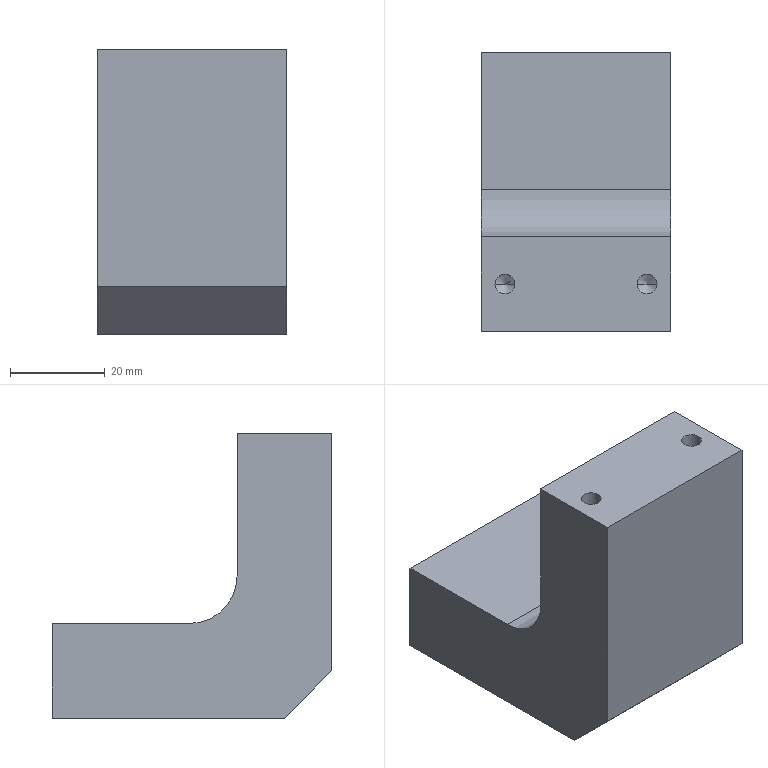Part | SolidWorks | features 3DProfileFeature 2, HoleWzd 2, Chamfer 1, Extrusion 1, Fillet 1, ICE 1 | 1 solid | 26 faces | box 40 x 59 x 60 mm | volume 77348 mm3 | cylinder 9 | plane 9 | cone 8 | commonest cylinder face diameters 4.2 x8 20 x1
STEP:
#1=CARTESIAN_POINT('',(-17.1,10.,17.6));
#2=VERTEX_POINT('',#1);
#3=CARTESIAN_POINT('',(-12.9,10.,17.6));
#4=VERTEX_POINT('',#3);
#5=CARTESIAN_POINT('',(-15.,10.,17.6));
#6=DIRECTION('',(0.,0.,1.));
#7=DIRECTION('',(1.,0.,0.));
#8=AXIS2_PLACEMENT_3D('',#5,#6,#7);
#9=CIRCLE('',#8,2.1);
#10=EDGE_CURVE('',#2,#4,#9,.T.);
#11=ORIENTED_EDGE('',*,*,#10,.F.);
#12=CARTESIAN_POINT('',(-17.1,10.,30.));
#13=VERTEX_POINT('',#12);
#14=CARTESIAN_POINT('',(-17.1,10.,30.));
#15=DIRECTION('',(0.,0.,1.));
#16=VECTOR('',#15,1000.);
#17=LINE('',#14,#16);
#18=EDGE_CURVE('',#2,#13,#17,.T.);
#19=ORIENTED_EDGE('',*,*,#18,.T.);
#20=CARTESIAN_POINT('',(-12.9,10.,30.));
#21=VERTEX_POINT('',#20);
#22=CARTESIAN_POINT('',(-15.,10.,30.));
#23=DIRECTION('',(0.,0.,1.));
#24=DIRECTION('',(1.,0.,0.));
#25=AXIS2_PLACEMENT_3D('',#22,#23,#24);
#26=CIRCLE('',#25,2.1);
#27=EDGE_CURVE('',#13,#21,#26,.T.);
#28=ORIENTED_EDGE('',*,*,#27,.T.);
#29=CARTESIAN_POINT('',(-12.9,10.,30.));
#30=DIRECTION('',(0.,0.,1.));
#31=VECTOR('',#30,1000.);
#32=LINE('',#29,#31);
#33=EDGE_CURVE('',#4,#21,#32,.T.);
#34=ORIENTED_EDGE('',*,*,#33,.F.);
#35=EDGE_LOOP('',(#11,#19,#28,#34));
#36=FACE_OUTER_BOUND('',#35,.T.);
#37=CARTESIAN_POINT('',(-15.,10.,30.));
#38=DIRECTION('',(0.,0.,1.));
#39=DIRECTION('',(1.,0.,0.));
#40=AXIS2_PLACEMENT_3D('',#37,#38,#39);
#41=CYLINDRICAL_SURFACE('',#40,2.1);
#42=ADVANCED_FACE('',(#36),#41,.F.);
#43=CARTESIAN_POINT('',(-15.,10.,16.338));
#44=VERTEX_POINT('',#43);
#45=CARTESIAN_POINT('',(-12.9,10.,17.6));
#46=DIRECTION('',(0.8572,0.,0.515));
#47=VECTOR('',#46,1000.);
#48=LINE('',#45,#47);
#49=EDGE_CURVE('',#44,#4,#48,.T.);
#50=ORIENTED_EDGE('',*,*,#49,.F.);
#51=CARTESIAN_POINT('',(-17.1,10.,17.6));
#52=DIRECTION('',(-0.8572,0.,0.515));
#53=VECTOR('',#52,1000.);
#54=LINE('',#51,#53);
#55=EDGE_CURVE('',#44,#2,#54,.T.);
#56=ORIENTED_EDGE('',*,*,#55,.T.);
#57=ORIENTED_EDGE('',*,*,#10,.T.);
#58=EDGE_LOOP('',(#50,#56,#57));
#59=FACE_OUTER_BOUND('',#58,.T.);
#60=CARTESIAN_POINT('',(-15.,10.,17.6));
#61=DIRECTION('',(0.,0.,1.));
#62=DIRECTION('',(1.,0.,0.));
#63=AXIS2_PLACEMENT_3D('',#60,#61,#62);
#64=CONICAL_SURFACE('',#63,2.1,1.03);
#65=ADVANCED_FACE('',(#59),#64,.F.);
#66=CARTESIAN_POINT('',(12.9,10.,17.6));
#67=VERTEX_POINT('',#66);
#68=CARTESIAN_POINT('',(17.1,10.,17.6));
#69=VERTEX_POINT('',#68);
#70=CARTESIAN_POINT('',(15.,10.,17.6));
#71=DIRECTION('',(0.,0.,1.));
#72=DIRECTION('',(1.,0.,0.));
#73=AXIS2_PLACEMENT_3D('',#70,#71,#72);
#74=CIRCLE('',#73,2.1);
#75=EDGE_CURVE('',#67,#69,#74,.T.);
#76=ORIENTED_EDGE('',*,*,#75,.F.);
#77=CARTESIAN_POINT('',(12.9,10.,30.));
#78=VERTEX_POINT('',#77);
#79=CARTESIAN_POINT('',(12.9,10.,30.));
#80=DIRECTION('',(0.,0.,1.));
#81=VECTOR('',#80,1000.);
#82=LINE('',#79,#81);
#83=EDGE_CURVE('',#67,#78,#82,.T.);
#84=ORIENTED_EDGE('',*,*,#83,.T.);
#85=CARTESIAN_POINT('',(17.1,10.,30.));
#86=VERTEX_POINT('',#85);
#87=CARTESIAN_POINT('',(15.,10.,30.));
#88=DIRECTION('',(0.,0.,1.));
#89=DIRECTION('',(1.,0.,0.));
#90=AXIS2_PLACEMENT_3D('',#87,#88,#89);
#91=CIRCLE('',#90,2.1);
#92=EDGE_CURVE('',#78,#86,#91,.T.);
#93=ORIENTED_EDGE('',*,*,#92,.T.);
#94=CARTESIAN_POINT('',(17.1,10.,30.));
#95=DIRECTION('',(0.,0.,1.));
#96=VECTOR('',#95,1000.);
#97=LINE('',#94,#96);
#98=EDGE_CURVE('',#69,#86,#97,.T.);
#99=ORIENTED_EDGE('',*,*,#98,.F.);
#100=EDGE_LOOP('',(#76,#84,#93,#99));
#101=FACE_OUTER_BOUND('',#100,.T.);
#102=CARTESIAN_POINT('',(15.,10.,30.));
#103=DIRECTION('',(0.,0.,1.));
#104=DIRECTION('',(1.,0.,0.));
#105=AXIS2_PLACEMENT_3D('',#102,#103,#104);
#106=CYLINDRICAL_SURFACE('',#105,2.1);
#107=ADVANCED_FACE('',(#101),#106,.F.);
#108=CARTESIAN_POINT('',(15.,10.,16.338));
#109=VERTEX_POINT('',#108);
#110=CARTESIAN_POINT('',(17.1,10.,17.6));
#111=DIRECTION('',(0.8572,0.,0.515));
#112=VECTOR('',#111,1000.);
#113=LINE('',#110,#112);
#114=EDGE_CURVE('',#109,#69,#113,.T.);
#115=ORIENTED_EDGE('',*,*,#114,.F.);
#116=CARTESIAN_POINT('',(12.9,10.,17.6));
#117=DIRECTION('',(-0.8572,0.,0.515));
#118=VECTOR('',#117,1000.);
#119=LINE('',#116,#118);
#120=EDGE_CURVE('',#109,#67,#119,.T.);
#121=ORIENTED_EDGE('',*,*,#120,.T.);
#122=ORIENTED_EDGE('',*,*,#75,.T.);
#123=EDGE_LOOP('',(#115,#121,#122));
#124=FACE_OUTER_BOUND('',#123,.T.);
#125=CARTESIAN_POINT('',(15.,10.,17.6));
#126=DIRECTION('',(0.,0.,1.));
#127=DIRECTION('',(1.,0.,0.));
#128=AXIS2_PLACEMENT_3D('',#125,#126,#127);
#129=CONICAL_SURFACE('',#128,2.1,1.03);
#130=ADVANCED_FACE('',(#124),#129,.F.);
#131=CARTESIAN_POINT('',(-14.,46.6,-22.1));
#132=VERTEX_POINT('',#131);
#133=CARTESIAN_POINT('',(-14.,46.6,-17.9));
#134=VERTEX_POINT('',#133);
#135=CARTESIAN_POINT('',(-14.,46.6,-20.));
#136=DIRECTION('',(0.,1.,0.));
#137=DIRECTION('',(0.,0.,1.));
#138=AXIS2_PLACEMENT_3D('',#135,#136,#137);
#139=CIRCLE('',#138,2.1);
#140=EDGE_CURVE('',#132,#134,#139,.T.);
#141=ORIENTED_EDGE('',*,*,#140,.F.);
#142=CARTESIAN_POINT('',(-14.,59.,-22.1));
#143=VERTEX_POINT('',#142);
#144=CARTESIAN_POINT('',(-14.,59.,-22.1));
#145=DIRECTION('',(0.,1.,0.));
#146=VECTOR('',#145,1000.);
#147=LINE('',#144,#146);
#148=EDGE_CURVE('',#132,#143,#147,.T.);
#149=ORIENTED_EDGE('',*,*,#148,.T.);
#150=CARTESIAN_POINT('',(-14.,59.,-17.9));
#151=VERTEX_POINT('',#150);
#152=CARTESIAN_POINT('',(-14.,59.,-20.));
#153=DIRECTION('',(0.,1.,0.));
#154=DIRECTION('',(0.,0.,1.));
#155=AXIS2_PLACEMENT_3D('',#152,#153,#154);
#156=CIRCLE('',#155,2.1);
#157=EDGE_CURVE('',#143,#151,#156,.T.);
#158=ORIENTED_EDGE('',*,*,#157,.T.);
#159=CARTESIAN_POINT('',(-14.,59.,-17.9));
#160=DIRECTION('',(0.,1.,0.));
#161=VECTOR('',#160,1000.);
#162=LINE('',#159,#161);
#163=EDGE_CURVE('',#134,#151,#162,.T.);
#164=ORIENTED_EDGE('',*,*,#163,.F.);
#165=EDGE_LOOP('',(#141,#149,#158,#164));
#166=FACE_OUTER_BOUND('',#165,.T.);
#167=CARTESIAN_POINT('',(-14.,59.,-20.));
#168=DIRECTION('',(0.,1.,0.));
#169=DIRECTION('',(0.,0.,1.));
#170=AXIS2_PLACEMENT_3D('',#167,#168,#169);
#171=CYLINDRICAL_SURFACE('',#170,2.1);
#172=ADVANCED_FACE('',(#166),#171,.F.);
#173=CARTESIAN_POINT('',(-14.,45.338,-20.));
#174=VERTEX_POINT('',#173);
#175=CARTESIAN_POINT('',(-14.,46.6,-17.9));
#176=DIRECTION('',(0.,0.515,0.8572));
#177=VECTOR('',#176,1000.);
#178=LINE('',#175,#177);
#179=EDGE_CURVE('',#174,#134,#178,.T.);
#180=ORIENTED_EDGE('',*,*,#179,.F.);
#181=CARTESIAN_POINT('',(-14.,46.6,-22.1));
#182=DIRECTION('',(0.,0.515,-0.8572));
#183=VECTOR('',#182,1000.);
#184=LINE('',#181,#183);
#185=EDGE_CURVE('',#174,#132,#184,.T.);
#186=ORIENTED_EDGE('',*,*,#185,.T.);
#187=ORIENTED_EDGE('',*,*,#140,.T.);
#188=EDGE_LOOP('',(#180,#186,#187));
#189=FACE_OUTER_BOUND('',#188,.T.);
#190=CARTESIAN_POINT('',(-14.,46.6,-20.));
#191=DIRECTION('',(0.,1.,0.));
#192=DIRECTION('',(0.,0.,1.));
#193=AXIS2_PLACEMENT_3D('',#190,#191,#192);
#194=CONICAL_SURFACE('',#193,2.1,1.03);
#195=ADVANCED_FACE('',(#189),#194,.F.);
#196=CARTESIAN_POINT('',(14.,46.6,-22.1));
#197=VERTEX_POINT('',#196);
#198=CARTESIAN_POINT('',(14.,46.6,-17.9));
#199=VERTEX_POINT('',#198);
#200=CARTESIAN_POINT('',(14.,46.6,-20.));
#201=DIRECTION('',(0.,1.,0.));
#202=DIRECTION('',(0.,0.,1.));
#203=AXIS2_PLACEMENT_3D('',#200,#201,#202);
#204=CIRCLE('',#203,2.1);
#205=EDGE_CURVE('',#197,#199,#204,.T.);
#206=ORIENTED_EDGE('',*,*,#205,.F.);
#207=CARTESIAN_POINT('',(14.,59.,-22.1));
#208=VERTEX_POINT('',#207);
#209=CARTESIAN_POINT('',(14.,59.,-22.1));
#210=DIRECTION('',(0.,1.,0.));
#211=VECTOR('',#210,1000.);
#212=LINE('',#209,#211);
#213=EDGE_CURVE('',#197,#208,#212,.T.);
#214=ORIENTED_EDGE('',*,*,#213,.T.);
#215=CARTESIAN_POINT('',(14.,59.,-17.9));
#216=VERTEX_POINT('',#215);
#217=CARTESIAN_POINT('',(14.,59.,-20.));
#218=DIRECTION('',(0.,1.,0.));
#219=DIRECTION('',(0.,0.,1.));
#220=AXIS2_PLACEMENT_3D('',#217,#218,#219);
#221=CIRCLE('',#220,2.1);
#222=EDGE_CURVE('',#208,#216,#221,.T.);
#223=ORIENTED_EDGE('',*,*,#222,.T.);
#224=CARTESIAN_POINT('',(14.,59.,-17.9));
#225=DIRECTION('',(0.,1.,0.));
#226=VECTOR('',#225,1000.);
#227=LINE('',#224,#226);
#228=EDGE_CURVE('',#199,#216,#227,.T.);
#229=ORIENTED_EDGE('',*,*,#228,.F.);
#230=EDGE_LOOP('',(#206,#214,#223,#229));
#231=FACE_OUTER_BOUND('',#230,.T.);
#232=CARTESIAN_POINT('',(14.,59.,-20.));
#233=DIRECTION('',(0.,1.,0.));
#234=DIRECTION('',(0.,0.,1.));
#235=AXIS2_PLACEMENT_3D('',#232,#233,#234);
#236=CYLINDRICAL_SURFACE('',#235,2.1);
#237=ADVANCED_FACE('',(#231),#236,.F.);
#238=CARTESIAN_POINT('',(14.,45.338,-20.));
#239=VERTEX_POINT('',#238);
#240=CARTESIAN_POINT('',(14.,46.6,-17.9));
#241=DIRECTION('',(0.,0.515,0.8572));
#242=VECTOR('',#241,1000.);
#243=LINE('',#240,#242);
#244=EDGE_CURVE('',#239,#199,#243,.T.);
#245=ORIENTED_EDGE('',*,*,#244,.F.);
#246=CARTESIAN_POINT('',(14.,46.6,-22.1));
#247=DIRECTION('',(0.,0.515,-0.8572));
#248=VECTOR('',#247,1000.);
#249=LINE('',#246,#248);
#250=EDGE_CURVE('',#239,#197,#249,.T.);
#251=ORIENTED_EDGE('',*,*,#250,.T.);
#252=ORIENTED_EDGE('',*,*,#205,.T.);
#253=EDGE_LOOP('',(#245,#251,#252));
#254=FACE_OUTER_BOUND('',#253,.T.);
#255=CARTESIAN_POINT('',(14.,46.6,-20.));
#256=DIRECTION('',(0.,1.,0.));
#257=DIRECTION('',(0.,0.,1.));
#258=AXIS2_PLACEMENT_3D('',#255,#256,#257);
#259=CONICAL_SURFACE('',#258,2.1,1.03);
#260=ADVANCED_FACE('',(#254),#259,.F.);
#261=CARTESIAN_POINT('',(20.,0.,30.));
#262=VERTEX_POINT('',#261);
#263=CARTESIAN_POINT('',(20.,0.,-20.));
#264=VERTEX_POINT('',#263);
#265=CARTESIAN_POINT('',(20.,0.,-30.));
#266=DIRECTION('',(0.,0.,-1.));
#267=VECTOR('',#266,1000.);
#268=LINE('',#265,#267);
#269=EDGE_CURVE('',#262,#264,#268,.T.);
#270=ORIENTED_EDGE('',*,*,#269,.T.);
#271=CARTESIAN_POINT('',(20.,10.,-30.));
#272=VERTEX_POINT('',#271);
#273=CARTESIAN_POINT('',(20.,10.,-30.));
#274=DIRECTION('',(0.,0.7071,-0.7071));
#275=VECTOR('',#274,1000.);
#276=LINE('',#273,#275);
#277=EDGE_CURVE('',#264,#272,#276,.T.);
#278=ORIENTED_EDGE('',*,*,#277,.T.);
#279=CARTESIAN_POINT('',(20.,59.,-30.));
#280=VERTEX_POINT('',#279);
#281=CARTESIAN_POINT('',(20.,59.,-30.));
#282=DIRECTION('',(0.,-1.,0.));
#283=VECTOR('',#282,1000.);
#284=LINE('',#281,#283);
#285=EDGE_CURVE('',#280,#272,#284,.T.);
#286=ORIENTED_EDGE('',*,*,#285,.F.);
#287=CARTESIAN_POINT('',(20.,59.,-10.));
#288=VERTEX_POINT('',#287);
#289=CARTESIAN_POINT('',(20.,59.,-30.));
#290=DIRECTION('',(0.,0.,-1.));
#291=VECTOR('',#290,1000.);
#292=LINE('',#289,#291);
#293=EDGE_CURVE('',#288,#280,#292,.T.);
#294=ORIENTED_EDGE('',*,*,#293,.F.);
#295=CARTESIAN_POINT('',(20.,30.,-10.));
#296=VERTEX_POINT('',#295);
#297=CARTESIAN_POINT('',(20.,59.,-10.));
#298=DIRECTION('',(0.,1.,0.));
#299=VECTOR('',#298,1000.);
#300=LINE('',#297,#299);
#301=EDGE_CURVE('',#296,#288,#300,.T.);
#302=ORIENTED_EDGE('',*,*,#301,.F.);
#303=CARTESIAN_POINT('',(20.,20.,0.));
#304=VERTEX_POINT('',#303);
#305=CARTESIAN_POINT('',(20.,30.,0.));
#306=DIRECTION('',(-1.,0.,0.));
#307=DIRECTION('',(0.,0.,1.));
#308=AXIS2_PLACEMENT_3D('',#305,#306,#307);
#309=CIRCLE('',#308,10.);
#310=EDGE_CURVE('',#296,#304,#309,.T.);
#311=ORIENTED_EDGE('',*,*,#310,.T.);
#312=CARTESIAN_POINT('',(20.,20.,30.));
#313=VERTEX_POINT('',#312);
#314=CARTESIAN_POINT('',(20.,20.,30.));
#315=DIRECTION('',(0.,0.,-1.));
#316=VECTOR('',#315,1000.);
#317=LINE('',#314,#316);
#318=EDGE_CURVE('',#313,#304,#317,.T.);
#319=ORIENTED_EDGE('',*,*,#318,.F.);
#320=CARTESIAN_POINT('',(20.,59.,30.));
#321=DIRECTION('',(0.,-1.,0.));
#322=VECTOR('',#321,1000.);
#323=LINE('',#320,#322);
#324=EDGE_CURVE('',#313,#262,#323,.T.);
#325=ORIENTED_EDGE('',*,*,#324,.T.);
#326=EDGE_LOOP('',(#270,#278,#286,#294,#302,#311,#319,#325));
#327=FACE_OUTER_BOUND('',#326,.T.);
#328=CARTESIAN_POINT('',(20.,59.,-30.));
#329=DIRECTION('',(-1.,0.,0.));
#330=DIRECTION('',(0.,0.,1.));
#331=AXIS2_PLACEMENT_3D('',#328,#329,#330);
#332=PLANE('',#331);
#333=ADVANCED_FACE('',(#327),#332,.F.);
#334=ORIENTED_EDGE('',*,*,#285,.T.);
#335=CARTESIAN_POINT('',(-20.,10.,-30.));
#336=VERTEX_POINT('',#335);
#337=CARTESIAN_POINT('',(-20.,10.,-30.));
#338=DIRECTION('',(-1.,0.,0.));
#339=VECTOR('',#338,1000.);
#340=LINE('',#337,#339);
#341=EDGE_CURVE('',#272,#336,#340,.T.);
#342=ORIENTED_EDGE('',*,*,#341,.T.);
#343=CARTESIAN_POINT('',(-20.,59.,-30.));
#344=VERTEX_POINT('',#343);
#345=CARTESIAN_POINT('',(-20.,59.,-30.));
#346=DIRECTION('',(0.,-1.,0.));
#347=VECTOR('',#346,1000.);
#348=LINE('',#345,#347);
#349=EDGE_CURVE('',#344,#336,#348,.T.);
#350=ORIENTED_EDGE('',*,*,#349,.F.);
#351=CARTESIAN_POINT('',(-20.,59.,-30.));
#352=DIRECTION('',(-1.,0.,0.));
#353=VECTOR('',#352,1000.);
#354=LINE('',#351,#353);
#355=EDGE_CURVE('',#280,#344,#354,.T.);
#356=ORIENTED_EDGE('',*,*,#355,.F.);
#357=EDGE_LOOP('',(#334,#342,#350,#356));
#358=FACE_OUTER_BOUND('',#357,.T.);
#359=CARTESIAN_POINT('',(-20.,59.,-30.));
#360=DIRECTION('',(0.,0.,1.));
#361=DIRECTION('',(1.,0.,0.));
#362=AXIS2_PLACEMENT_3D('',#359,#360,#361);
#363=PLANE('',#362);
#364=ADVANCED_FACE('',(#358),#363,.F.);
#365=ORIENTED_EDGE('',*,*,#349,.T.);
#366=CARTESIAN_POINT('',(-20.,0.,-20.));
#367=VERTEX_POINT('',#366);
#368=CARTESIAN_POINT('',(-20.,10.,-30.));
#369=DIRECTION('',(0.,-0.7071,0.7071));
#370=VECTOR('',#369,1000.);
#371=LINE('',#368,#370);
#372=EDGE_CURVE('',#336,#367,#371,.T.);
#373=ORIENTED_EDGE('',*,*,#372,.T.);
#374=CARTESIAN_POINT('',(-20.,0.,30.));
#375=VERTEX_POINT('',#374);
#376=CARTESIAN_POINT('',(-20.,0.,-30.));
#377=DIRECTION('',(0.,0.,1.));
#378=VECTOR('',#377,1000.);
#379=LINE('',#376,#378);
#380=EDGE_CURVE('',#367,#375,#379,.T.);
#381=ORIENTED_EDGE('',*,*,#380,.T.);
#382=CARTESIAN_POINT('',(-20.,20.,30.));
#383=VERTEX_POINT('',#382);
#384=CARTESIAN_POINT('',(-20.,59.,30.));
#385=DIRECTION('',(0.,-1.,0.));
#386=VECTOR('',#385,1000.);
#387=LINE('',#384,#386);
#388=EDGE_CURVE('',#383,#375,#387,.T.);
#389=ORIENTED_EDGE('',*,*,#388,.F.);
#390=CARTESIAN_POINT('',(-20.,20.,0.));
#391=VERTEX_POINT('',#390);
#392=CARTESIAN_POINT('',(-20.,20.,-30.));
#393=DIRECTION('',(0.,0.,-1.));
#394=VECTOR('',#393,1000.);
#395=LINE('',#392,#394);
#396=EDGE_CURVE('',#383,#391,#395,.T.);
#397=ORIENTED_EDGE('',*,*,#396,.T.);
#398=CARTESIAN_POINT('',(-20.,30.,-10.));
#399=VERTEX_POINT('',#398);
#400=CARTESIAN_POINT('',(-20.,30.,0.));
#401=DIRECTION('',(1.,0.,0.));
#402=DIRECTION('',(0.,0.,-1.));
#403=AXIS2_PLACEMENT_3D('',#400,#401,#402);
#404=CIRCLE('',#403,10.);
#405=EDGE_CURVE('',#391,#399,#404,.T.);
#406=ORIENTED_EDGE('',*,*,#405,.T.);
#407=CARTESIAN_POINT('',(-20.,59.,-10.));
#408=VERTEX_POINT('',#407);
#409=CARTESIAN_POINT('',(-20.,59.,-10.));
#410=DIRECTION('',(0.,1.,0.));
#411=VECTOR('',#410,1000.);
#412=LINE('',#409,#411);
#413=EDGE_CURVE('',#399,#408,#412,.T.);
#414=ORIENTED_EDGE('',*,*,#413,.T.);
#415=CARTESIAN_POINT('',(-20.,59.,-30.));
#416=DIRECTION('',(0.,0.,1.));
#417=VECTOR('',#416,1000.);
#418=LINE('',#415,#417);
#419=EDGE_CURVE('',#344,#408,#418,.T.);
#420=ORIENTED_EDGE('',*,*,#419,.F.);
#421=EDGE_LOOP('',(#365,#373,#381,#389,#397,#406,#414,#420));
#422=FACE_OUTER_BOUND('',#421,.T.);
#423=CARTESIAN_POINT('',(-20.,59.,-30.));
#424=DIRECTION('',(1.,0.,0.));
#425=DIRECTION('',(0.,0.,-1.));
#426=AXIS2_PLACEMENT_3D('',#423,#424,#425);
#427=PLANE('',#426);
#428=ADVANCED_FACE('',(#422),#427,.F.);
#429=CARTESIAN_POINT('',(-15.,10.,30.));
#430=DIRECTION('',(0.,0.,1.));
#431=DIRECTION('',(1.,0.,0.));
#432=AXIS2_PLACEMENT_3D('',#429,#430,#431);
#433=CIRCLE('',#432,2.1);
#434=EDGE_CURVE('',#21,#13,#433,.T.);
#435=ORIENTED_EDGE('',*,*,#434,.F.);
#436=ORIENTED_EDGE('',*,*,#27,.F.);
#437=EDGE_LOOP('',(#435,#436));
#438=FACE_BOUND('',#437,.T.);
#439=CARTESIAN_POINT('',(15.,10.,30.));
#440=DIRECTION('',(0.,0.,1.));
#441=DIRECTION('',(1.,0.,0.));
#442=AXIS2_PLACEMENT_3D('',#439,#440,#441);
#443=CIRCLE('',#442,2.1);
#444=EDGE_CURVE('',#86,#78,#443,.T.);
#445=ORIENTED_EDGE('',*,*,#444,.F.);
#446=ORIENTED_EDGE('',*,*,#92,.F.);
#447=EDGE_LOOP('',(#445,#446));
#448=FACE_BOUND('',#447,.T.);
#449=ORIENTED_EDGE('',*,*,#324,.F.);
#450=CARTESIAN_POINT('',(-25.,20.,30.));
#451=DIRECTION('',(1.,0.,0.));
#452=VECTOR('',#451,1000.);
#453=LINE('',#450,#452);
#454=EDGE_CURVE('',#383,#313,#453,.T.);
#455=ORIENTED_EDGE('',*,*,#454,.F.);
#456=ORIENTED_EDGE('',*,*,#388,.T.);
#457=CARTESIAN_POINT('',(-20.,0.,30.));
#458=DIRECTION('',(1.,0.,0.));
#459=VECTOR('',#458,1000.);
#460=LINE('',#457,#459);
#461=EDGE_CURVE('',#375,#262,#460,.T.);
#462=ORIENTED_EDGE('',*,*,#461,.T.);
#463=EDGE_LOOP('',(#449,#455,#456,#462));
#464=FACE_OUTER_BOUND('',#463,.T.);
#465=CARTESIAN_POINT('',(-20.,59.,30.));
#466=DIRECTION('',(0.,0.,-1.));
#467=DIRECTION('',(-1.,0.,0.));
#468=AXIS2_PLACEMENT_3D('',#465,#466,#467);
#469=PLANE('',#468);
#470=ADVANCED_FACE('',(#438,#448,#464),#469,.F.);
#471=CARTESIAN_POINT('',(-14.,59.,-20.));
#472=DIRECTION('',(0.,1.,0.));
#473=DIRECTION('',(0.,0.,1.));
#474=AXIS2_PLACEMENT_3D('',#471,#472,#473);
#475=CIRCLE('',#474,2.1);
#476=EDGE_CURVE('',#151,#143,#475,.T.);
#477=ORIENTED_EDGE('',*,*,#476,.F.);
#478=ORIENTED_EDGE('',*,*,#157,.F.);
#479=EDGE_LOOP('',(#477,#478));
#480=FACE_BOUND('',#479,.T.);
#481=CARTESIAN_POINT('',(14.,59.,-20.));
#482=DIRECTION('',(0.,1.,0.));
#483=DIRECTION('',(0.,0.,1.));
#484=AXIS2_PLACEMENT_3D('',#481,#482,#483);
#485=CIRCLE('',#484,2.1);
#486=EDGE_CURVE('',#216,#208,#485,.T.);
#487=ORIENTED_EDGE('',*,*,#486,.F.);
#488=ORIENTED_EDGE('',*,*,#222,.F.);
#489=EDGE_LOOP('',(#487,#488));
#490=FACE_BOUND('',#489,.T.);
#491=CARTESIAN_POINT('',(0.,59.,-10.));
#492=DIRECTION('',(-1.,0.,0.));
#493=VECTOR('',#492,1000.);
#494=LINE('',#491,#493);
#495=EDGE_CURVE('',#288,#408,#494,.T.);
#496=ORIENTED_EDGE('',*,*,#495,.F.);
#497=ORIENTED_EDGE('',*,*,#293,.T.);
#498=ORIENTED_EDGE('',*,*,#355,.T.);
#499=ORIENTED_EDGE('',*,*,#419,.T.);
#500=EDGE_LOOP('',(#496,#497,#498,#499));
#501=FACE_OUTER_BOUND('',#500,.T.);
#502=CARTESIAN_POINT('',(0.,59.,0.));
#503=DIRECTION('',(0.,1.,0.));
#504=DIRECTION('',(0.,0.,1.));
#505=AXIS2_PLACEMENT_3D('',#502,#503,#504);
#506=PLANE('',#505);
#507=ADVANCED_FACE('',(#480,#490,#501),#506,.T.);
#508=ORIENTED_EDGE('',*,*,#380,.F.);
#509=CARTESIAN_POINT('',(0.,0.,-20.));
#510=DIRECTION('',(1.,0.,0.));
#511=VECTOR('',#510,1000.);
#512=LINE('',#509,#511);
#513=EDGE_CURVE('',#367,#264,#512,.T.);
#514=ORIENTED_EDGE('',*,*,#513,.T.);
#515=ORIENTED_EDGE('',*,*,#269,.F.);
#516=ORIENTED_EDGE('',*,*,#461,.F.);
#517=EDGE_LOOP('',(#508,#514,#515,#516));
#518=FACE_OUTER_BOUND('',#517,.T.);
#519=CARTESIAN_POINT('',(0.,0.,0.));
#520=DIRECTION('',(0.,1.,0.));
#521=DIRECTION('',(0.,0.,1.));
#522=AXIS2_PLACEMENT_3D('',#519,#520,#521);
#523=PLANE('',#522);
#524=ADVANCED_FACE('',(#518),#523,.F.);
#525=ORIENTED_EDGE('',*,*,#318,.T.);
#526=CARTESIAN_POINT('',(-20.,20.,0.));
#527=DIRECTION('',(-1.,0.,0.));
#528=VECTOR('',#527,1000.);
#529=LINE('',#526,#528);
#530=EDGE_CURVE('',#304,#391,#529,.T.);
#531=ORIENTED_EDGE('',*,*,#530,.T.);
#532=ORIENTED_EDGE('',*,*,#396,.F.);
#533=ORIENTED_EDGE('',*,*,#454,.T.);
#534=EDGE_LOOP('',(#525,#531,#532,#533));
#535=FACE_OUTER_BOUND('',#534,.T.);
#536=CARTESIAN_POINT('',(-25.,20.,30.));
#537=DIRECTION('',(0.,-1.,0.));
#538=DIRECTION('',(0.,0.,-1.));
#539=AXIS2_PLACEMENT_3D('',#536,#537,#538);
#540=PLANE('',#539);
#541=ADVANCED_FACE('',(#535),#540,.F.);
#542=ORIENTED_EDGE('',*,*,#413,.F.);
#543=CARTESIAN_POINT('',(20.,30.,-10.));
#544=DIRECTION('',(1.,0.,0.));
#545=VECTOR('',#544,1000.);
#546=LINE('',#543,#545);
#547=EDGE_CURVE('',#399,#296,#546,.T.);
#548=ORIENTED_EDGE('',*,*,#547,.T.);
#549=ORIENTED_EDGE('',*,*,#301,.T.);
#550=ORIENTED_EDGE('',*,*,#495,.T.);
#551=EDGE_LOOP('',(#542,#548,#549,#550));
#552=FACE_OUTER_BOUND('',#551,.T.);
#553=CARTESIAN_POINT('',(-25.,59.,-10.));
#554=DIRECTION('',(0.,0.,-1.));
#555=DIRECTION('',(-1.,0.,0.));
#556=AXIS2_PLACEMENT_3D('',#553,#554,#555);
#557=PLANE('',#556);
#558=ADVANCED_FACE('',(#552),#557,.F.);
#559=ORIENTED_EDGE('',*,*,#277,.F.);
#560=ORIENTED_EDGE('',*,*,#513,.F.);
#561=ORIENTED_EDGE('',*,*,#372,.F.);
#562=ORIENTED_EDGE('',*,*,#341,.F.);
#563=EDGE_LOOP('',(#559,#560,#561,#562));
#564=FACE_OUTER_BOUND('',#563,.T.);
#565=CARTESIAN_POINT('',(-20.,10.,-30.));
#566=DIRECTION('',(0.,0.7071,0.7071));
#567=DIRECTION('',(-1.,0.,0.));
#568=AXIS2_PLACEMENT_3D('',#565,#566,#567);
#569=PLANE('',#568);
#570=ADVANCED_FACE('',(#564),#569,.F.);
#571=ORIENTED_EDGE('',*,*,#405,.F.);
#572=ORIENTED_EDGE('',*,*,#530,.F.);
#573=ORIENTED_EDGE('',*,*,#310,.F.);
#574=ORIENTED_EDGE('',*,*,#547,.F.);
#575=EDGE_LOOP('',(#571,#572,#573,#574));
#576=FACE_OUTER_BOUND('',#575,.T.);
#577=CARTESIAN_POINT('',(-25.,30.,0.));
#578=DIRECTION('',(-1.,0.,0.));
#579=DIRECTION('',(0.,0.,1.));
#580=AXIS2_PLACEMENT_3D('',#577,#578,#579);
#581=CYLINDRICAL_SURFACE('',#580,10.);
#582=ADVANCED_FACE('',(#576),#581,.F.);
#583=ORIENTED_EDGE('',*,*,#250,.F.);
#584=ORIENTED_EDGE('',*,*,#244,.T.);
#585=CARTESIAN_POINT('',(14.,46.6,-20.));
#586=DIRECTION('',(0.,1.,0.));
#587=DIRECTION('',(0.,0.,1.));
#588=AXIS2_PLACEMENT_3D('',#585,#586,#587);
#589=CIRCLE('',#588,2.1);
#590=EDGE_CURVE('',#199,#197,#589,.T.);
#591=ORIENTED_EDGE('',*,*,#590,.T.);
#592=EDGE_LOOP('',(#583,#584,#591));
#593=FACE_OUTER_BOUND('',#592,.T.);
#594=CARTESIAN_POINT('',(14.,46.6,-20.));
#595=DIRECTION('',(0.,1.,0.));
#596=DIRECTION('',(0.,0.,1.));
#597=AXIS2_PLACEMENT_3D('',#594,#595,#596);
#598=CONICAL_SURFACE('',#597,2.1,1.03);
#599=ADVANCED_FACE('',(#593),#598,.F.);
#600=ORIENTED_EDGE('',*,*,#213,.F.);
#601=ORIENTED_EDGE('',*,*,#590,.F.);
#602=ORIENTED_EDGE('',*,*,#228,.T.);
#603=ORIENTED_EDGE('',*,*,#486,.T.);
#604=EDGE_LOOP('',(#600,#601,#602,#603));
#605=FACE_OUTER_BOUND('',#604,.T.);
#606=CARTESIAN_POINT('',(14.,59.,-20.));
#607=DIRECTION('',(0.,1.,0.));
#608=DIRECTION('',(0.,0.,1.));
#609=AXIS2_PLACEMENT_3D('',#606,#607,#608);
#610=CYLINDRICAL_SURFACE('',#609,2.1);
#611=ADVANCED_FACE('',(#605),#610,.F.);
#612=ORIENTED_EDGE('',*,*,#185,.F.);
#613=ORIENTED_EDGE('',*,*,#179,.T.);
#614=CARTESIAN_POINT('',(-14.,46.6,-20.));
#615=DIRECTION('',(0.,1.,0.));
#616=DIRECTION('',(0.,0.,1.));
#617=AXIS2_PLACEMENT_3D('',#614,#615,#616);
#618=CIRCLE('',#617,2.1);
#619=EDGE_CURVE('',#134,#132,#618,.T.);
#620=ORIENTED_EDGE('',*,*,#619,.T.);
#621=EDGE_LOOP('',(#612,#613,#620));
#622=FACE_OUTER_BOUND('',#621,.T.);
#623=CARTESIAN_POINT('',(-14.,46.6,-20.));
#624=DIRECTION('',(0.,1.,0.));
#625=DIRECTION('',(0.,0.,1.));
#626=AXIS2_PLACEMENT_3D('',#623,#624,#625);
#627=CONICAL_SURFACE('',#626,2.1,1.03);
#628=ADVANCED_FACE('',(#622),#627,.F.);
#629=ORIENTED_EDGE('',*,*,#148,.F.);
#630=ORIENTED_EDGE('',*,*,#619,.F.);
#631=ORIENTED_EDGE('',*,*,#163,.T.);
#632=ORIENTED_EDGE('',*,*,#476,.T.);
#633=EDGE_LOOP('',(#629,#630,#631,#632));
#634=FACE_OUTER_BOUND('',#633,.T.);
#635=CARTESIAN_POINT('',(-14.,59.,-20.));
#636=DIRECTION('',(0.,1.,0.));
#637=DIRECTION('',(0.,0.,1.));
#638=AXIS2_PLACEMENT_3D('',#635,#636,#637);
#639=CYLINDRICAL_SURFACE('',#638,2.1);
#640=ADVANCED_FACE('',(#634),#639,.F.);
#641=ORIENTED_EDGE('',*,*,#120,.F.);
#642=ORIENTED_EDGE('',*,*,#114,.T.);
#643=CARTESIAN_POINT('',(15.,10.,17.6));
#644=DIRECTION('',(0.,0.,1.));
#645=DIRECTION('',(1.,0.,0.));
#646=AXIS2_PLACEMENT_3D('',#643,#644,#645);
#647=CIRCLE('',#646,2.1);
#648=EDGE_CURVE('',#69,#67,#647,.T.);
#649=ORIENTED_EDGE('',*,*,#648,.T.);
#650=EDGE_LOOP('',(#641,#642,#649));
#651=FACE_OUTER_BOUND('',#650,.T.);
#652=CARTESIAN_POINT('',(15.,10.,17.6));
#653=DIRECTION('',(0.,0.,1.));
#654=DIRECTION('',(1.,0.,0.));
#655=AXIS2_PLACEMENT_3D('',#652,#653,#654);
#656=CONICAL_SURFACE('',#655,2.1,1.03);
#657=ADVANCED_FACE('',(#651),#656,.F.);
#658=ORIENTED_EDGE('',*,*,#83,.F.);
#659=ORIENTED_EDGE('',*,*,#648,.F.);
#660=ORIENTED_EDGE('',*,*,#98,.T.);
#661=ORIENTED_EDGE('',*,*,#444,.T.);
#662=EDGE_LOOP('',(#658,#659,#660,#661));
#663=FACE_OUTER_BOUND('',#662,.T.);
#664=CARTESIAN_POINT('',(15.,10.,30.));
#665=DIRECTION('',(0.,0.,1.));
#666=DIRECTION('',(1.,0.,0.));
#667=AXIS2_PLACEMENT_3D('',#664,#665,#666);
#668=CYLINDRICAL_SURFACE('',#667,2.1);
#669=ADVANCED_FACE('',(#663),#668,.F.);
#670=ORIENTED_EDGE('',*,*,#55,.F.);
#671=ORIENTED_EDGE('',*,*,#49,.T.);
#672=CARTESIAN_POINT('',(-15.,10.,17.6));
#673=DIRECTION('',(0.,0.,1.));
#674=DIRECTION('',(1.,0.,0.));
#675=AXIS2_PLACEMENT_3D('',#672,#673,#674);
#676=CIRCLE('',#675,2.1);
#677=EDGE_CURVE('',#4,#2,#676,.T.);
#678=ORIENTED_EDGE('',*,*,#677,.T.);
#679=EDGE_LOOP('',(#670,#671,#678));
#680=FACE_OUTER_BOUND('',#679,.T.);
#681=CARTESIAN_POINT('',(-15.,10.,17.6));
#682=DIRECTION('',(0.,0.,1.));
#683=DIRECTION('',(1.,0.,0.));
#684=AXIS2_PLACEMENT_3D('',#681,#682,#683);
#685=CONICAL_SURFACE('',#684,2.1,1.03);
#686=ADVANCED_FACE('',(#680),#685,.F.);
#687=ORIENTED_EDGE('',*,*,#18,.F.);
#688=ORIENTED_EDGE('',*,*,#677,.F.);
#689=ORIENTED_EDGE('',*,*,#33,.T.);
#690=ORIENTED_EDGE('',*,*,#434,.T.);
#691=EDGE_LOOP('',(#687,#688,#689,#690));
#692=FACE_OUTER_BOUND('',#691,.T.);
#693=CARTESIAN_POINT('',(-15.,10.,30.));
#694=DIRECTION('',(0.,0.,1.));
#695=DIRECTION('',(1.,0.,0.));
#696=AXIS2_PLACEMENT_3D('',#693,#694,#695);
#697=CYLINDRICAL_SURFACE('',#696,2.1);
#698=ADVANCED_FACE('',(#692),#697,.F.);
#699=CLOSED_SHELL('',(#42,#65,#107,#130,#172,#195,#237,#260,#333,#364,#428,#470,#507,#524,#541,#558,#570,#582,#599,#611,#628,#640,#657,#669,#686,#698));
#700=MANIFOLD_SOLID_BREP('',#699);
#701=CARTESIAN_POINT('',(0.,0.,0.));
#702=DIRECTION('',(0.,0.,1.));
#703=DIRECTION('',(1.,0.,0.));
#704=AXIS2_PLACEMENT_3D('',#701,#702,#703);
#705=(LENGTH_UNIT()NAMED_UNIT(*)SI_UNIT(.MILLI.,.METRE.));
#706=UNCERTAINTY_MEASURE_WITH_UNIT(LENGTH_MEASURE(0.00001),#705,'','');
#707=(NAMED_UNIT(*)PLANE_ANGLE_UNIT()SI_UNIT($,.RADIAN.));
#708=(NAMED_UNIT(*)SI_UNIT($,.STERADIAN.)SOLID_ANGLE_UNIT());
#709=(GEOMETRIC_REPRESENTATION_CONTEXT(3)GLOBAL_UNCERTAINTY_ASSIGNED_CONTEXT((#706))GLOBAL_UNIT_ASSIGNED_CONTEXT((#705,#707,#708))REPRESENTATION_CONTEXT('',''));
#710=ADVANCED_BREP_SHAPE_REPRESENTATION('',(#700,#704),#709);